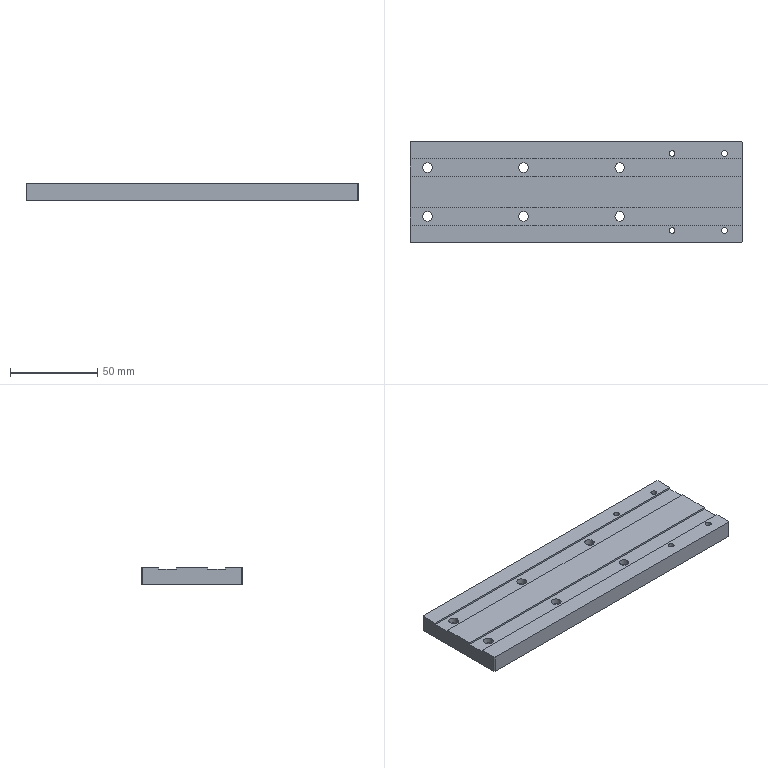Part | STEP file | PN_0091 Mount electronic clip connecting plate B | 1 solid | 62 faces | box 190 x 58 x 10 mm | volume 99887 mm3 | cylinder 34 | plane 28 | commonest cylinder face diameters 5.5 x12 10 x12 3.3 x8 5 x2